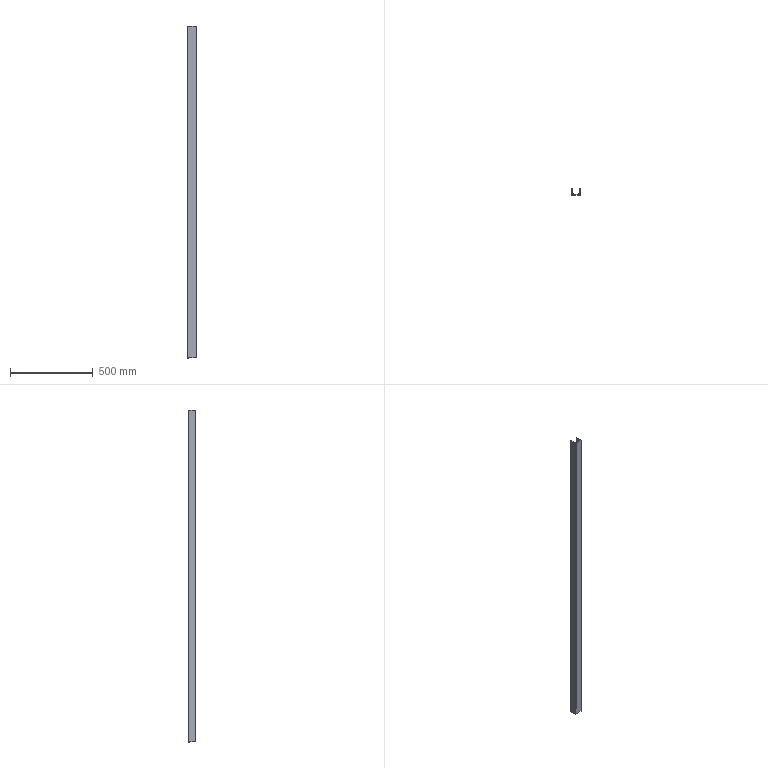Part | SolidWorks | features Extrusion 1 | 1 solid | 12 faces | box 50 x 37 x 2000 mm | volume 1093372 mm3 | plane 8 | cylinder 4 | commonest cylinder face diameters 7 x2 14 x2
STEP:
#1=CARTESIAN_POINT('',(-25.,37.,-1000.));
#2=VERTEX_POINT('',#1);
#3=CARTESIAN_POINT('',(-25.,0.,-1000.));
#4=VERTEX_POINT('',#3);
#5=CARTESIAN_POINT('',(-25.,0.,-1000.));
#6=DIRECTION('',(0.,-1.,0.));
#7=VECTOR('',#6,1000.);
#8=LINE('',#5,#7);
#9=EDGE_CURVE('',#2,#4,#8,.T.);
#10=ORIENTED_EDGE('',*,*,#9,.T.);
#11=CARTESIAN_POINT('',(-25.,0.,1000.));
#12=VERTEX_POINT('',#11);
#13=CARTESIAN_POINT('',(-25.,0.,1000.));
#14=DIRECTION('',(0.,0.,-1.));
#15=VECTOR('',#14,1000.);
#16=LINE('',#13,#15);
#17=EDGE_CURVE('',#12,#4,#16,.T.);
#18=ORIENTED_EDGE('',*,*,#17,.F.);
#19=CARTESIAN_POINT('',(-25.,37.,1000.));
#20=VERTEX_POINT('',#19);
#21=CARTESIAN_POINT('',(-25.,0.,1000.));
#22=DIRECTION('',(0.,-1.,0.));
#23=VECTOR('',#22,1000.);
#24=LINE('',#21,#23);
#25=EDGE_CURVE('',#20,#12,#24,.T.);
#26=ORIENTED_EDGE('',*,*,#25,.F.);
#27=CARTESIAN_POINT('',(-25.,37.,1000.));
#28=DIRECTION('',(0.,0.,-1.));
#29=VECTOR('',#28,1000.);
#30=LINE('',#27,#29);
#31=EDGE_CURVE('',#20,#2,#30,.T.);
#32=ORIENTED_EDGE('',*,*,#31,.T.);
#33=EDGE_LOOP('',(#10,#18,#26,#32));
#34=FACE_OUTER_BOUND('',#33,.T.);
#35=CARTESIAN_POINT('',(-25.,0.,1000.));
#36=DIRECTION('',(1.,0.,0.));
#37=DIRECTION('',(0.,1.,0.));
#38=AXIS2_PLACEMENT_3D('',#35,#36,#37);
#39=PLANE('',#38);
#40=ADVANCED_FACE('',(#34),#39,.F.);
#41=CARTESIAN_POINT('',(25.,0.,-1000.));
#42=VERTEX_POINT('',#41);
#43=CARTESIAN_POINT('',(-25.,0.,-1000.));
#44=DIRECTION('',(1.,0.,0.));
#45=VECTOR('',#44,1000.);
#46=LINE('',#43,#45);
#47=EDGE_CURVE('',#4,#42,#46,.T.);
#48=ORIENTED_EDGE('',*,*,#47,.T.);
#49=CARTESIAN_POINT('',(25.,0.,1000.));
#50=VERTEX_POINT('',#49);
#51=CARTESIAN_POINT('',(25.,0.,1000.));
#52=DIRECTION('',(0.,0.,-1.));
#53=VECTOR('',#52,1000.);
#54=LINE('',#51,#53);
#55=EDGE_CURVE('',#50,#42,#54,.T.);
#56=ORIENTED_EDGE('',*,*,#55,.F.);
#57=CARTESIAN_POINT('',(-25.,0.,1000.));
#58=DIRECTION('',(1.,0.,0.));
#59=VECTOR('',#58,1000.);
#60=LINE('',#57,#59);
#61=EDGE_CURVE('',#12,#50,#60,.T.);
#62=ORIENTED_EDGE('',*,*,#61,.F.);
#63=ORIENTED_EDGE('',*,*,#17,.T.);
#64=EDGE_LOOP('',(#48,#56,#62,#63));
#65=FACE_OUTER_BOUND('',#64,.T.);
#66=CARTESIAN_POINT('',(-25.,0.,1000.));
#67=DIRECTION('',(0.,1.,0.));
#68=DIRECTION('',(-1.,0.,0.));
#69=AXIS2_PLACEMENT_3D('',#66,#67,#68);
#70=PLANE('',#69);
#71=ADVANCED_FACE('',(#65),#70,.F.);
#72=CARTESIAN_POINT('',(25.,37.,-1000.));
#73=VERTEX_POINT('',#72);
#74=CARTESIAN_POINT('',(25.,0.,-1000.));
#75=DIRECTION('',(0.,1.,0.));
#76=VECTOR('',#75,1000.);
#77=LINE('',#74,#76);
#78=EDGE_CURVE('',#42,#73,#77,.T.);
#79=ORIENTED_EDGE('',*,*,#78,.T.);
#80=CARTESIAN_POINT('',(25.,37.,1000.));
#81=VERTEX_POINT('',#80);
#82=CARTESIAN_POINT('',(25.,37.,1000.));
#83=DIRECTION('',(0.,0.,-1.));
#84=VECTOR('',#83,1000.);
#85=LINE('',#82,#84);
#86=EDGE_CURVE('',#81,#73,#85,.T.);
#87=ORIENTED_EDGE('',*,*,#86,.F.);
#88=CARTESIAN_POINT('',(25.,0.,1000.));
#89=DIRECTION('',(0.,1.,0.));
#90=VECTOR('',#89,1000.);
#91=LINE('',#88,#90);
#92=EDGE_CURVE('',#50,#81,#91,.T.);
#93=ORIENTED_EDGE('',*,*,#92,.F.);
#94=ORIENTED_EDGE('',*,*,#55,.T.);
#95=EDGE_LOOP('',(#79,#87,#93,#94));
#96=FACE_OUTER_BOUND('',#95,.T.);
#97=CARTESIAN_POINT('',(25.,0.,1000.));
#98=DIRECTION('',(-1.,0.,0.));
#99=DIRECTION('',(0.,-1.,0.));
#100=AXIS2_PLACEMENT_3D('',#97,#98,#99);
#101=PLANE('',#100);
#102=ADVANCED_FACE('',(#96),#101,.F.);
#103=CARTESIAN_POINT('',(21.55,33.848,-1000.));
#104=VERTEX_POINT('',#103);
#105=CARTESIAN_POINT('',(25.033,33.5,-1000.));
#106=DIRECTION('',(0.,0.,1.));
#107=DIRECTION('',(-1.,0.,0.));
#108=AXIS2_PLACEMENT_3D('',#105,#106,#107);
#109=CIRCLE('',#108,3.5);
#110=EDGE_CURVE('',#73,#104,#109,.T.);
#111=ORIENTED_EDGE('',*,*,#110,.T.);
#112=CARTESIAN_POINT('',(21.55,33.848,1000.));
#113=VERTEX_POINT('',#112);
#114=CARTESIAN_POINT('',(21.55,33.848,1000.));
#115=DIRECTION('',(0.,0.,-1.));
#116=VECTOR('',#115,1000.);
#117=LINE('',#114,#116);
#118=EDGE_CURVE('',#113,#104,#117,.T.);
#119=ORIENTED_EDGE('',*,*,#118,.F.);
#120=CARTESIAN_POINT('',(25.033,33.5,1000.));
#121=DIRECTION('',(0.,0.,1.));
#122=DIRECTION('',(-1.,0.,0.));
#123=AXIS2_PLACEMENT_3D('',#120,#121,#122);
#124=CIRCLE('',#123,3.5);
#125=EDGE_CURVE('',#81,#113,#124,.T.);
#126=ORIENTED_EDGE('',*,*,#125,.F.);
#127=ORIENTED_EDGE('',*,*,#86,.T.);
#128=EDGE_LOOP('',(#111,#119,#126,#127));
#129=FACE_OUTER_BOUND('',#128,.T.);
#130=CARTESIAN_POINT('',(25.033,33.5,1000.));
#131=DIRECTION('',(0.,0.,-1.));
#132=DIRECTION('',(-1.,0.,0.));
#133=AXIS2_PLACEMENT_3D('',#130,#131,#132);
#134=CYLINDRICAL_SURFACE('',#133,3.5);
#135=ADVANCED_FACE('',(#129),#134,.T.);
#136=CARTESIAN_POINT('',(19.25,10.805,-1000.));
#137=VERTEX_POINT('',#136);
#138=CARTESIAN_POINT('',(21.55,33.848,-1000.));
#139=DIRECTION('',(-0.09932,-0.9951,0.));
#140=VECTOR('',#139,1000.);
#141=LINE('',#138,#140);
#142=EDGE_CURVE('',#104,#137,#141,.T.);
#143=ORIENTED_EDGE('',*,*,#142,.T.);
#144=CARTESIAN_POINT('',(19.25,10.805,1000.));
#145=VERTEX_POINT('',#144);
#146=CARTESIAN_POINT('',(19.25,10.805,1000.));
#147=DIRECTION('',(0.,0.,-1.));
#148=VECTOR('',#147,1000.);
#149=LINE('',#146,#148);
#150=EDGE_CURVE('',#145,#137,#149,.T.);
#151=ORIENTED_EDGE('',*,*,#150,.F.);
#152=CARTESIAN_POINT('',(21.55,33.848,1000.));
#153=DIRECTION('',(-0.09932,-0.9951,0.));
#154=VECTOR('',#153,1000.);
#155=LINE('',#152,#154);
#156=EDGE_CURVE('',#113,#145,#155,.T.);
#157=ORIENTED_EDGE('',*,*,#156,.F.);
#158=ORIENTED_EDGE('',*,*,#118,.T.);
#159=EDGE_LOOP('',(#143,#151,#157,#158));
#160=FACE_OUTER_BOUND('',#159,.T.);
#161=CARTESIAN_POINT('',(21.55,33.848,1000.));
#162=DIRECTION('',(0.9951,-0.09932,0.));
#163=DIRECTION('',(0.09932,0.9951,0.));
#164=AXIS2_PLACEMENT_3D('',#161,#162,#163);
#165=PLANE('',#164);
#166=ADVANCED_FACE('',(#160),#165,.F.);
#167=CARTESIAN_POINT('',(12.285,4.5,-1000.));
#168=VERTEX_POINT('',#167);
#169=CARTESIAN_POINT('',(12.285,11.5,-1000.));
#170=DIRECTION('',(0.,0.,-1.));
#171=DIRECTION('',(1.,0.,0.));
#172=AXIS2_PLACEMENT_3D('',#169,#170,#171);
#173=CIRCLE('',#172,7.);
#174=EDGE_CURVE('',#137,#168,#173,.T.);
#175=ORIENTED_EDGE('',*,*,#174,.T.);
#176=CARTESIAN_POINT('',(12.285,4.5,1000.));
#177=VERTEX_POINT('',#176);
#178=CARTESIAN_POINT('',(12.285,4.5,1000.));
#179=DIRECTION('',(0.,0.,-1.));
#180=VECTOR('',#179,1000.);
#181=LINE('',#178,#180);
#182=EDGE_CURVE('',#177,#168,#181,.T.);
#183=ORIENTED_EDGE('',*,*,#182,.F.);
#184=CARTESIAN_POINT('',(12.285,11.5,1000.));
#185=DIRECTION('',(0.,0.,-1.));
#186=DIRECTION('',(1.,0.,0.));
#187=AXIS2_PLACEMENT_3D('',#184,#185,#186);
#188=CIRCLE('',#187,7.);
#189=EDGE_CURVE('',#145,#177,#188,.T.);
#190=ORIENTED_EDGE('',*,*,#189,.F.);
#191=ORIENTED_EDGE('',*,*,#150,.T.);
#192=EDGE_LOOP('',(#175,#183,#190,#191));
#193=FACE_OUTER_BOUND('',#192,.T.);
#194=CARTESIAN_POINT('',(12.285,11.5,1000.));
#195=DIRECTION('',(0.,0.,-1.));
#196=DIRECTION('',(-1.,0.,0.));
#197=AXIS2_PLACEMENT_3D('',#194,#195,#196);
#198=CYLINDRICAL_SURFACE('',#197,7.);
#199=ADVANCED_FACE('',(#193),#198,.F.);
#200=CARTESIAN_POINT('',(-12.285,4.5,-1000.));
#201=VERTEX_POINT('',#200);
#202=CARTESIAN_POINT('',(-12.285,4.5,-1000.));
#203=DIRECTION('',(-1.,0.,0.));
#204=VECTOR('',#203,1000.);
#205=LINE('',#202,#204);
#206=EDGE_CURVE('',#168,#201,#205,.T.);
#207=ORIENTED_EDGE('',*,*,#206,.T.);
#208=CARTESIAN_POINT('',(-12.285,4.5,1000.));
#209=VERTEX_POINT('',#208);
#210=CARTESIAN_POINT('',(-12.285,4.5,1000.));
#211=DIRECTION('',(0.,0.,-1.));
#212=VECTOR('',#211,1000.);
#213=LINE('',#210,#212);
#214=EDGE_CURVE('',#209,#201,#213,.T.);
#215=ORIENTED_EDGE('',*,*,#214,.F.);
#216=CARTESIAN_POINT('',(-12.285,4.5,1000.));
#217=DIRECTION('',(-1.,0.,0.));
#218=VECTOR('',#217,1000.);
#219=LINE('',#216,#218);
#220=EDGE_CURVE('',#177,#209,#219,.T.);
#221=ORIENTED_EDGE('',*,*,#220,.F.);
#222=ORIENTED_EDGE('',*,*,#182,.T.);
#223=EDGE_LOOP('',(#207,#215,#221,#222));
#224=FACE_OUTER_BOUND('',#223,.T.);
#225=CARTESIAN_POINT('',(-12.285,4.5,1000.));
#226=DIRECTION('',(0.,-1.,0.));
#227=DIRECTION('',(0.,0.,-1.));
#228=AXIS2_PLACEMENT_3D('',#225,#226,#227);
#229=PLANE('',#228);
#230=ADVANCED_FACE('',(#224),#229,.F.);
#231=CARTESIAN_POINT('',(-19.25,10.805,-1000.));
#232=VERTEX_POINT('',#231);
#233=CARTESIAN_POINT('',(-12.285,11.5,-1000.));
#234=DIRECTION('',(0.,0.,-1.));
#235=DIRECTION('',(-1.,0.,0.));
#236=AXIS2_PLACEMENT_3D('',#233,#234,#235);
#237=CIRCLE('',#236,7.);
#238=EDGE_CURVE('',#201,#232,#237,.T.);
#239=ORIENTED_EDGE('',*,*,#238,.T.);
#240=CARTESIAN_POINT('',(-19.25,10.805,1000.));
#241=VERTEX_POINT('',#240);
#242=CARTESIAN_POINT('',(-19.25,10.805,1000.));
#243=DIRECTION('',(0.,0.,-1.));
#244=VECTOR('',#243,1000.);
#245=LINE('',#242,#244);
#246=EDGE_CURVE('',#241,#232,#245,.T.);
#247=ORIENTED_EDGE('',*,*,#246,.F.);
#248=CARTESIAN_POINT('',(-12.285,11.5,1000.));
#249=DIRECTION('',(0.,0.,-1.));
#250=DIRECTION('',(-1.,0.,0.));
#251=AXIS2_PLACEMENT_3D('',#248,#249,#250);
#252=CIRCLE('',#251,7.);
#253=EDGE_CURVE('',#209,#241,#252,.T.);
#254=ORIENTED_EDGE('',*,*,#253,.F.);
#255=ORIENTED_EDGE('',*,*,#214,.T.);
#256=EDGE_LOOP('',(#239,#247,#254,#255));
#257=FACE_OUTER_BOUND('',#256,.T.);
#258=CARTESIAN_POINT('',(-12.285,11.5,1000.));
#259=DIRECTION('',(0.,0.,-1.));
#260=DIRECTION('',(-1.,0.,0.));
#261=AXIS2_PLACEMENT_3D('',#258,#259,#260);
#262=CYLINDRICAL_SURFACE('',#261,7.);
#263=ADVANCED_FACE('',(#257),#262,.F.);
#264=CARTESIAN_POINT('',(-21.55,33.848,-1000.));
#265=VERTEX_POINT('',#264);
#266=CARTESIAN_POINT('',(-21.55,33.848,-1000.));
#267=DIRECTION('',(-0.09932,0.9951,0.));
#268=VECTOR('',#267,1000.);
#269=LINE('',#266,#268);
#270=EDGE_CURVE('',#232,#265,#269,.T.);
#271=ORIENTED_EDGE('',*,*,#270,.T.);
#272=CARTESIAN_POINT('',(-21.55,33.848,1000.));
#273=VERTEX_POINT('',#272);
#274=CARTESIAN_POINT('',(-21.55,33.848,1000.));
#275=DIRECTION('',(0.,0.,-1.));
#276=VECTOR('',#275,1000.);
#277=LINE('',#274,#276);
#278=EDGE_CURVE('',#273,#265,#277,.T.);
#279=ORIENTED_EDGE('',*,*,#278,.F.);
#280=CARTESIAN_POINT('',(-21.55,33.848,1000.));
#281=DIRECTION('',(-0.09932,0.9951,0.));
#282=VECTOR('',#281,1000.);
#283=LINE('',#280,#282);
#284=EDGE_CURVE('',#241,#273,#283,.T.);
#285=ORIENTED_EDGE('',*,*,#284,.F.);
#286=ORIENTED_EDGE('',*,*,#246,.T.);
#287=EDGE_LOOP('',(#271,#279,#285,#286));
#288=FACE_OUTER_BOUND('',#287,.T.);
#289=CARTESIAN_POINT('',(-21.55,33.848,1000.));
#290=DIRECTION('',(-0.9951,-0.09932,0.));
#291=DIRECTION('',(0.09932,-0.9951,0.));
#292=AXIS2_PLACEMENT_3D('',#289,#290,#291);
#293=PLANE('',#292);
#294=ADVANCED_FACE('',(#288),#293,.F.);
#295=CARTESIAN_POINT('',(-25.033,33.5,-1000.));
#296=DIRECTION('',(0.,0.,1.));
#297=DIRECTION('',(1.,0.,0.));
#298=AXIS2_PLACEMENT_3D('',#295,#296,#297);
#299=CIRCLE('',#298,3.5);
#300=EDGE_CURVE('',#265,#2,#299,.T.);
#301=ORIENTED_EDGE('',*,*,#300,.T.);
#302=ORIENTED_EDGE('',*,*,#31,.F.);
#303=CARTESIAN_POINT('',(-25.033,33.5,1000.));
#304=DIRECTION('',(0.,0.,1.));
#305=DIRECTION('',(1.,0.,0.));
#306=AXIS2_PLACEMENT_3D('',#303,#304,#305);
#307=CIRCLE('',#306,3.5);
#308=EDGE_CURVE('',#273,#20,#307,.T.);
#309=ORIENTED_EDGE('',*,*,#308,.F.);
#310=ORIENTED_EDGE('',*,*,#278,.T.);
#311=EDGE_LOOP('',(#301,#302,#309,#310));
#312=FACE_OUTER_BOUND('',#311,.T.);
#313=CARTESIAN_POINT('',(-25.033,33.5,1000.));
#314=DIRECTION('',(0.,0.,-1.));
#315=DIRECTION('',(-1.,0.,0.));
#316=AXIS2_PLACEMENT_3D('',#313,#314,#315);
#317=CYLINDRICAL_SURFACE('',#316,3.5);
#318=ADVANCED_FACE('',(#312),#317,.T.);
#319=ORIENTED_EDGE('',*,*,#25,.T.);
#320=ORIENTED_EDGE('',*,*,#61,.T.);
#321=ORIENTED_EDGE('',*,*,#92,.T.);
#322=ORIENTED_EDGE('',*,*,#125,.T.);
#323=ORIENTED_EDGE('',*,*,#156,.T.);
#324=ORIENTED_EDGE('',*,*,#189,.T.);
#325=ORIENTED_EDGE('',*,*,#220,.T.);
#326=ORIENTED_EDGE('',*,*,#253,.T.);
#327=ORIENTED_EDGE('',*,*,#284,.T.);
#328=ORIENTED_EDGE('',*,*,#308,.T.);
#329=EDGE_LOOP('',(#319,#320,#321,#322,#323,#324,#325,#326,#327,#328));
#330=FACE_OUTER_BOUND('',#329,.T.);
#331=CARTESIAN_POINT('',(-25.033,33.5,1000.));
#332=DIRECTION('',(0.,0.,1.));
#333=DIRECTION('',(1.,0.,0.));
#334=AXIS2_PLACEMENT_3D('',#331,#332,#333);
#335=PLANE('',#334);
#336=ADVANCED_FACE('',(#330),#335,.T.);
#337=ORIENTED_EDGE('',*,*,#9,.F.);
#338=ORIENTED_EDGE('',*,*,#300,.F.);
#339=ORIENTED_EDGE('',*,*,#270,.F.);
#340=ORIENTED_EDGE('',*,*,#238,.F.);
#341=ORIENTED_EDGE('',*,*,#206,.F.);
#342=ORIENTED_EDGE('',*,*,#174,.F.);
#343=ORIENTED_EDGE('',*,*,#142,.F.);
#344=ORIENTED_EDGE('',*,*,#110,.F.);
#345=ORIENTED_EDGE('',*,*,#78,.F.);
#346=ORIENTED_EDGE('',*,*,#47,.F.);
#347=EDGE_LOOP('',(#337,#338,#339,#340,#341,#342,#343,#344,#345,#346));
#348=FACE_OUTER_BOUND('',#347,.T.);
#349=CARTESIAN_POINT('',(-25.033,33.5,-1000.));
#350=DIRECTION('',(0.,0.,1.));
#351=DIRECTION('',(1.,0.,0.));
#352=AXIS2_PLACEMENT_3D('',#349,#350,#351);
#353=PLANE('',#352);
#354=ADVANCED_FACE('',(#348),#353,.F.);
#355=CLOSED_SHELL('',(#40,#71,#102,#135,#166,#199,#230,#263,#294,#318,#336,#354));
#356=MANIFOLD_SOLID_BREP('',#355);
#357=CARTESIAN_POINT('',(0.,0.,0.));
#358=DIRECTION('',(0.,0.,1.));
#359=DIRECTION('',(1.,0.,0.));
#360=AXIS2_PLACEMENT_3D('',#357,#358,#359);
#361=(LENGTH_UNIT()NAMED_UNIT(*)SI_UNIT(.MILLI.,.METRE.));
#362=UNCERTAINTY_MEASURE_WITH_UNIT(LENGTH_MEASURE(0.00001),#361,'','');
#363=(NAMED_UNIT(*)PLANE_ANGLE_UNIT()SI_UNIT($,.RADIAN.));
#364=(NAMED_UNIT(*)SI_UNIT($,.STERADIAN.)SOLID_ANGLE_UNIT());
#365=(GEOMETRIC_REPRESENTATION_CONTEXT(3)GLOBAL_UNCERTAINTY_ASSIGNED_CONTEXT((#362))GLOBAL_UNIT_ASSIGNED_CONTEXT((#361,#363,#364))REPRESENTATION_CONTEXT('',''));
#366=ADVANCED_BREP_SHAPE_REPRESENTATION('',(#356,#360),#365);